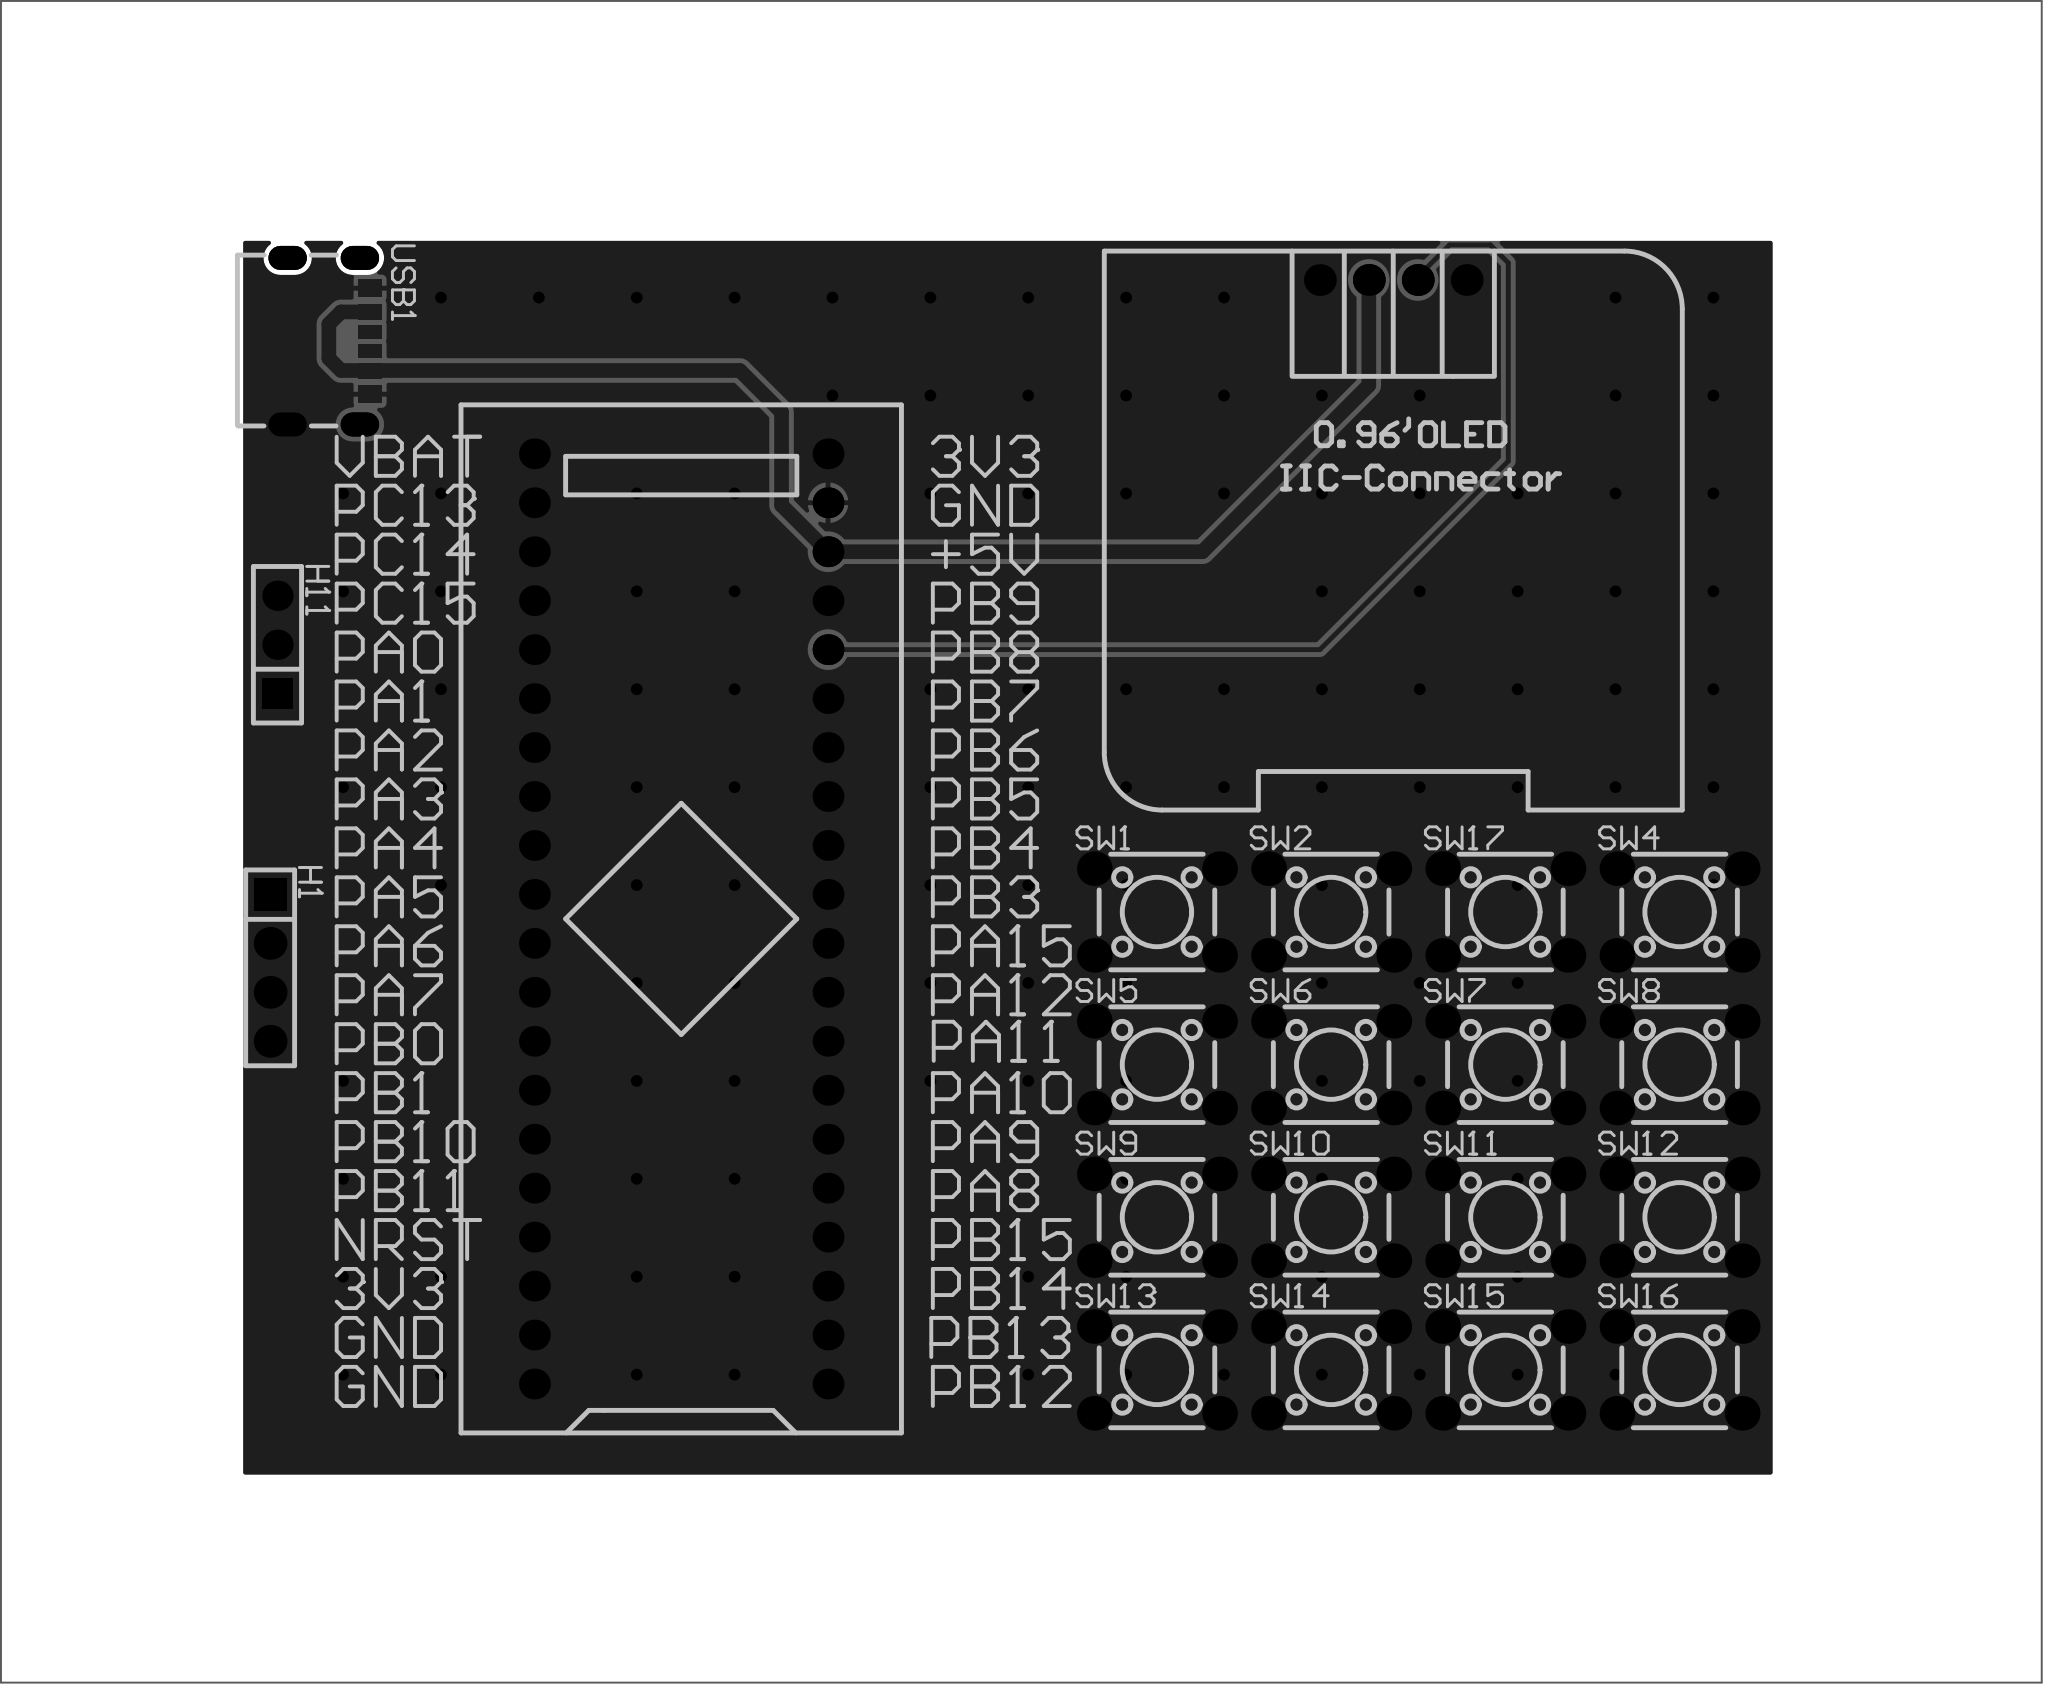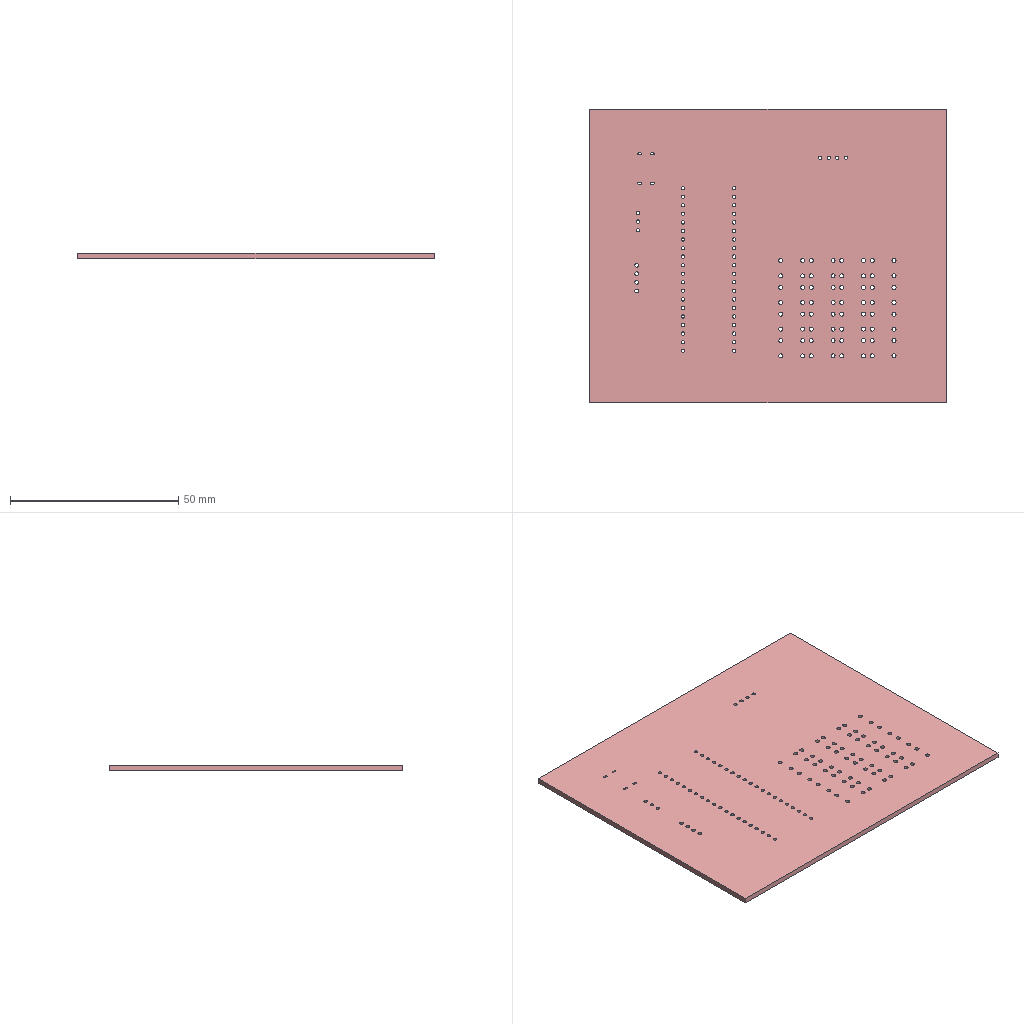Circuit board layout | Altium Designer | box 105.9 x 87.2 x 1.6 mm
Layer stack:
# Altium Designer layer stack of  (unit mm; dielectric type: 0 none, 1 core, 2 prepreg, 3 surface material)
index,name,kind,layer,copper_thickness_mm,dielectric_type,dielectric_thickness_mm,dielectric_material,dielectric_constant
0,Top Paste Mask Layer,other,,,,,,
1,Top Silkscreen Layer,other,,,,,,
2,Top Solder Mask Layer,dielectric,,,3,0.01,,3.3
3,Top Layer,copper,Top Layer,0.035,,,,
4,Dielectric1,dielectric,,,3,1.51,FR4,4.5
5,Bottom Layer,copper,Bottom Layer,0.035,,,,
6,Bottom Solder Mask Layer,dielectric,,,3,0.01,,3.3
7,Bottom Silkscreen Layer,other,,,,,,
8,Bottom Paste Mask Layer,other,,,,,,
# drill layer pairs: low layer,high layer
drill_pair,Top Layer,Bottom Layer
Part placement:
Designator,Comment,Layer,Footprint,Center-X(mm),Center-Y(mm),Rotation
SW6,KH-6X6X6H-TJ,TopLayer,SW-TH_4P-L6.0-W6.0-P4.50-LS6.5,138.889,101.912,0
SW2,KH-6X6X6H-TJ,TopLayer,SW-TH_4P-L6.0-W6.0-P4.50-LS6.5,138.889,109.831,0
SW10,KH-6X6X6H-TJ,TopLayer,SW-TH_4P-L6.0-W6.0-P4.50-LS6.5,138.889,93.993,0
SW7,KH-6X6X6H-TJ,TopLayer,SW-TH_4P-L6.0-W6.0-P4.50-LS6.5,147.93,101.912,0
SW11,KH-6X6X6H-TJ,TopLayer,SW-TH_4P-L6.0-W6.0-P4.50-LS6.5,147.93,93.993,0
SW17,KH-6X6X6H-TJ,TopLayer,SW-TH_4P-L6.0-W6.0-P4.50-LS6.5,147.93,109.831,0
SW1,KH-6X6X6H-TJ,TopLayer,SW-TH_4P-L6.0-W6.0-P4.50-LS6.5,129.847,109.831,0
SW13,KH-6X6X6H-TJ,TopLayer,SW-TH_4P-L6.0-W6.0-P4.50-LS6.5,129.847,86.073,0
SW5,KH-6X6X6H-TJ,TopLayer,SW-TH_4P-L6.0-W6.0-P4.50-LS6.5,129.847,101.912,0
SW9,KH-6X6X6H-TJ,TopLayer,SW-TH_4P-L6.0-W6.0-P4.50-LS6.5,129.847,93.993,0
SW14,KH-6X6X6H-TJ,TopLayer,SW-TH_4P-L6.0-W6.0-P4.50-LS6.5,138.889,86.073,0
SW15,KH-6X6X6H-TJ,TopLayer,SW-TH_4P-L6.0-W6.0-P4.50-LS6.5,147.93,86.073,0
SW4,KH-6X6X6H-TJ,TopLayer,SW-TH_4P-L6.0-W6.0-P4.50-LS6.5,156.972,109.831,0
SW12,KH-6X6X6H-TJ,TopLayer,SW-TH_4P-L6.0-W6.0-P4.50-LS6.5,156.972,93.993,0
SW16,KH-6X6X6H-TJ,TopLayer,SW-TH_4P-L6.0-W6.0-P4.50-LS6.5,156.972,86.073,0
SW8,KH-6X6X6H-TJ,TopLayer,SW-TH_4P-L6.0-W6.0-P4.50-LS6.5,156.972,101.912,0
U1,STM32F103C8T6-Card,TopLayer,CONN-TH_L53.3-W22.9_STM32F103C8T6-CARD,105.156,109.474,90
H11,,TopLayer,HDR-TH_3P-P2.54-V-F,84.201,123.698,90
OLED1,,TopLayer,0.96OLED_4P,142.113,142.621,0
H1,,TopLayer,HDR-TH_4P-P2.54-V-M,83.82,106.934,270
USB1,,TopLayer,USB__TYPE-C-6P,86.868,139.446,270
Pad and via stacks:
# Altium Designer via and pad stacks of  (unit mm). Each distinct definition once, with the count of objects using it.
# via: kind,start_layer,end_layer,hole_mm,diameter_mm,mode(0 simple;1 top-mid-bottom;2 full stack),diameter_per_layer,count,example_net
# pad: kind,layer,hole_mm,hole_type(0 round;1 square;2 slot),plating,top_size,top_shape(1 round;2 rect;3 octagon;9 rounded rect),mid_size,bottom_size,mode,footprint,size_per_layer,count,example
pad,Multi-Layer,1.2,0,plated,1.8x1.8,1,1.8x1.8,1.8x1.8,0,SW-TH_4P-L6.0-W6.0-P4.50-LS6.5,,64,SW6.1
pad,Multi-Layer,1,0,plated,1.6x1.6,1,1.6x1.6,1.6x1.6,0,CONN-TH_L53.3-W22.9_STM32F103C8T6-CARD,,40,U1.1
pad,Multi-Layer,1.02,0,plated,1.575x1.575,1,1.575x1.575,1.575x1.575,0,HDR-TH_3P-P2.54-V-F,,2,H11.3
pad,Multi-Layer,1.02,0,plated,1.575x1.575,2,1.575x1.575,1.575x1.575,0,HDR-TH_3P-P2.54-V-F,,1,H11.1
pad,Multi-Layer,1,0,plated,1.65x1.65,1,1.65x1.65,1.65x1.65,0,0.96OLED_4P,,4,OLED1.4
pad,Multi-Layer,1.1,0,plated,1.7x1.7,2,1.7x1.7,1.7x1.7,0,HDR-TH_4P-P2.54-V-M,,1,H1.1
pad,Multi-Layer,1.1,0,plated,1.7x1.7,1,1.7x1.7,1.7x1.7,0,HDR-TH_4P-P2.54-V-M,,3,H1.2
pad,Multi-Layer,0.6,2,plated,1.25x2,1,1.25x2,1.25x2,0,USB_ TYPE-C-6P,,4,USB1.8
pad,Top Layer,0,0,plated,0.7x1.2,2,0.7x1.2,0.7x1.2,0,USB_ TYPE-C-6P,,2,USB1.A5
pad,Top Layer,0,0,plated,0.8x1.2,2,0.8x1.2,0.8x1.2,0,USB_ TYPE-C-6P,,2,USB1.B9
pad,Top Layer,0,0,plated,0.9x1.2,2,0.9x1.2,0.9x1.2,0,USB_ TYPE-C-6P,,2,USB1.B12
via,Top Layer,Bottom Layer,0.3048,0.61,0,,118,GND
Copper pours:
name,layer,net,type(0 solid;1 hatched;2 none)
Top Layer-GND,Top Layer,GND,0
Bottom Layer-GND,Bottom Layer,GND,0